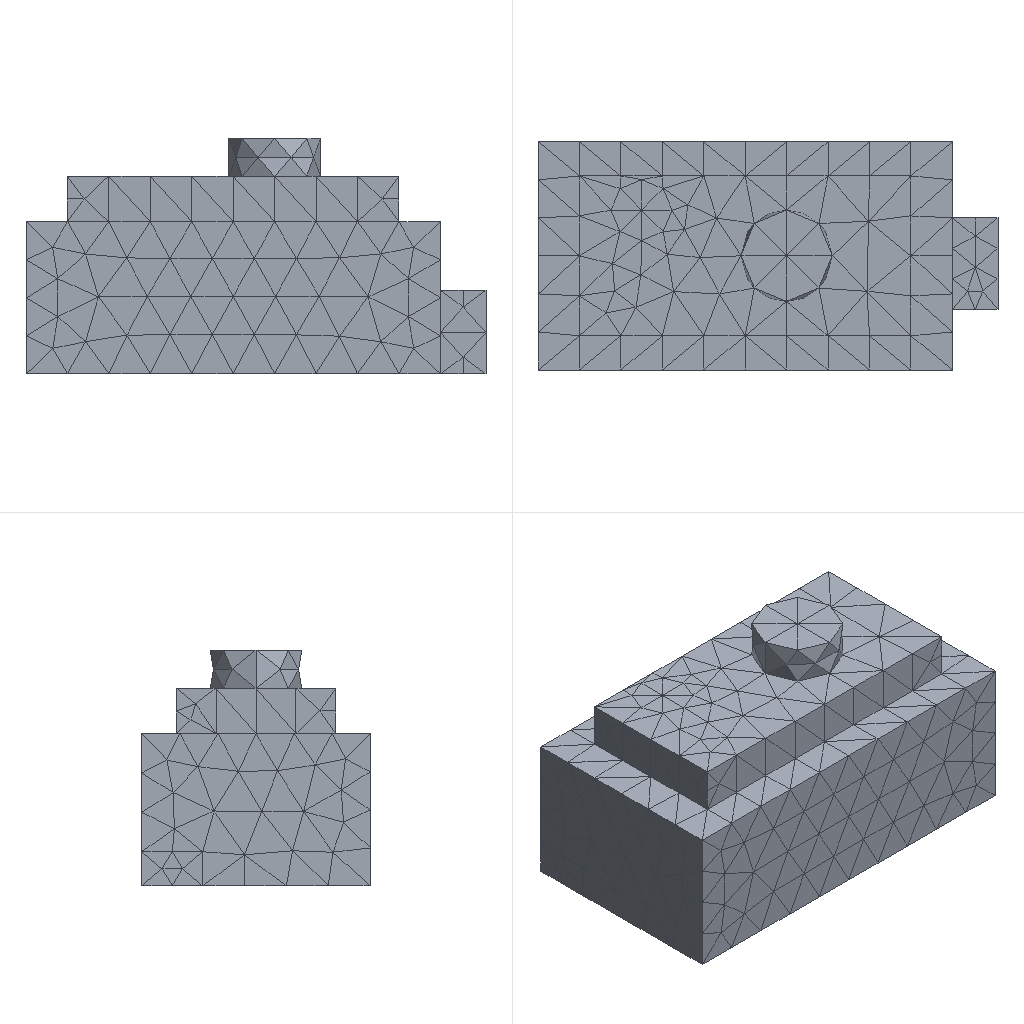Simulation study | ansys mapdl
Set-up summary:
category,name,step,type,value,unit,region
solver,ansys_mapdl
units,mm-N-s-tonne (MPa),,inferred,E=210000 density=
analysis,model,,static
mesh,nodes,,,3959
mesh,elements,,,2344
element_type,SOLID187,,,2344
material,mat 1,,E,210000
material,mat 1,,nu,0.3
load,,model,body load temp,,,all
load,,model,force,"1000 [dir=(0, 0, -1) n=308]",,node list
bc,,model,fixed,"[dofs=UX,UY,UZ n=4599]",,node list
Ansys APDL input file, long lists of numbers shortened:
/COM,ANSYS RELEASE 2026 R1           BUILD 26.1      UP20260202       09:09:58
/PREP7
/NOPR
/TITLE,2
ANTYPE, 0
*IF,_CDRDOFF,EQ,1,THEN     !if solid model was read in
_CDRDOFF=             !reset flag, numoffs already performed
*ELSE              !offset database for the following FE model
NUMOFF,NODE,     3959
NUMOFF,ELEM,     2344
NUMOFF,MAT ,        1
NUMOFF,TYPE,        1
*ENDIF
*SET,_RETURN ,  0.
*SET,_STATUS ,  0.
*SET,_UIQR   ,  308.
*SET,__FLOATPARAMETER__,  3959.
DOF,DELETE
ETBLOCK,        1,        1
(2i9,19a9)
        1      187        0        0        0        0        0        0        0        0        0        0        0        0        0        0        0        0        0        0        0
       -1
NBLOCK,6,SOLID,      3959,      3959
(3i9,6e21.13e3)
        1        0        0-3.8450000000000E+001 3.0000000000000E+001 9.0000000000000E+000
! (3958 more lines like these left out)
N,UNBL,LOC,       -1,
EBLOCK,19,SOLID,      2344,      2344
(19i10)
         1         1         1         1         0         0         0         0        10         0         1      1571      1572      1573      1574      1789      1790      1791      1792
! (4687 more lines like these left out)
        -1
MPTEMP,UNBL, 1, 1,  0.    ,
MPDATA,UNBL, 1,EX  ,       1, 1,  210000.000    ,
MPTEMP,UNBL, 1, 1,  0.    ,
MPDATA,UNBL, 1,NUXY,       1, 1, 0.3    ,
MPTEMP,UNBL, 1, 1,  0.    ,
MPDATA,UNBL, 1,PRXY,       1, 1, 0.3    ,
EXTOPT,ATTR,      0,      0,      0
EXTOPT,ESIZE,  0,  0.
EXTOPT,ACLEAR,      0
TREF,  0.
IRLF,  0
BFUNIF,TEMP,_TINY
ACEL,  0.    ,  0.    ,  0.
OMEGA,  0.    ,  0.    ,  0.
DOMEGA,  0.    ,  0.    ,  0.
CGLOC,  0.    ,  0.    ,  0.
CGOMEGA,  0.    ,  0.    ,  0.
DCGOMG,  0.    ,  0.    ,  0.
KUSE,     0
TIME,  0.
ALPHAD,  0.
BETAD,  0.
DMPRAT,  0.
DMPSTR,  0.
CRPLIM, 0.1    ,   0
CRPLIM,  0.    ,   1
NCNV,     0, 1.000000000E+12,     0,  0.    ,  0.
NEQIT,     0
ERESX,DEFA
DBLOCK,      4599
(i9,a6,2(pg16.9))
        1  UX    0.00000000      0.00000000
! (4598 more lines like these left out)
       -1
FBLOCK,       308
(i9,a6,2(pg16.9))
      521  FZ   -3.24675325      0.00000000
! (307 more lines like these left out)
       -1
/GO
FINISH
Results summary:
result,analysis_type_db,,,static,unstated
result,n_sets,,,1,unstated
result,load_steps[0].set,load_step=1,,1,unstated
result,load_steps[0].substep,load_step=1,,1,unstated
result,load_steps[0].time,load_step=1,,1,unstated
result,load_steps[0].freq,load_step=1,,1,unstated
result,load_steps[0].max_usum,load_step=1,,0.000115,unstated
result,load_steps[0].max_seqv,load_step=1,,1.086,unstated
result,load_steps[0].reaction_sum.FX,load_step=1,,1.03597e-11,unstated
result,load_steps[0].reaction_sum.FY,load_step=1,,5.33978e-12,unstated
result,load_steps[0].reaction_sum.FZ,load_step=1,,1000,unstated
result,load_steps[0].reaction_sum.MX,load_step=1,,0,unstated
result,load_steps[0].reaction_sum.MY,load_step=1,,0,unstated
result,load_steps[0].reaction_sum.MZ,load_step=1,,0,unstated
result,convergence,,,results present for all listed sets,unstated